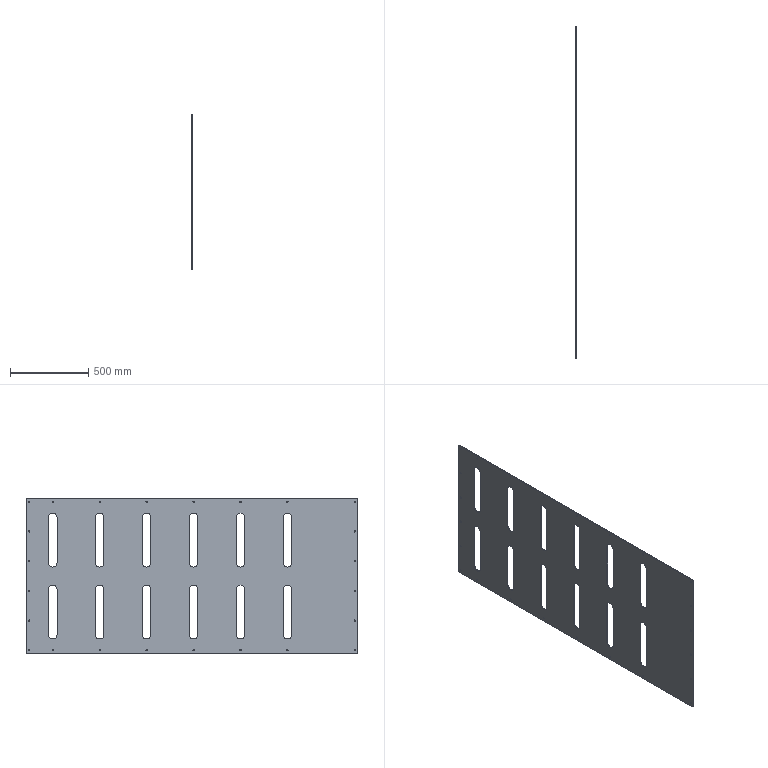Part | SolidWorks | features LPattern 7, ICE 5, MirrorPattern 4, Fillet 2, HoleWzd 2, Extrusion 1 | 1 solid | 118 faces | box 5 x 2120 x 990 mm | volume 9387989 mm3 | cylinder 88 | plane 30 | commonest cylinder face diameters 8 x48 55 x36 20 x4